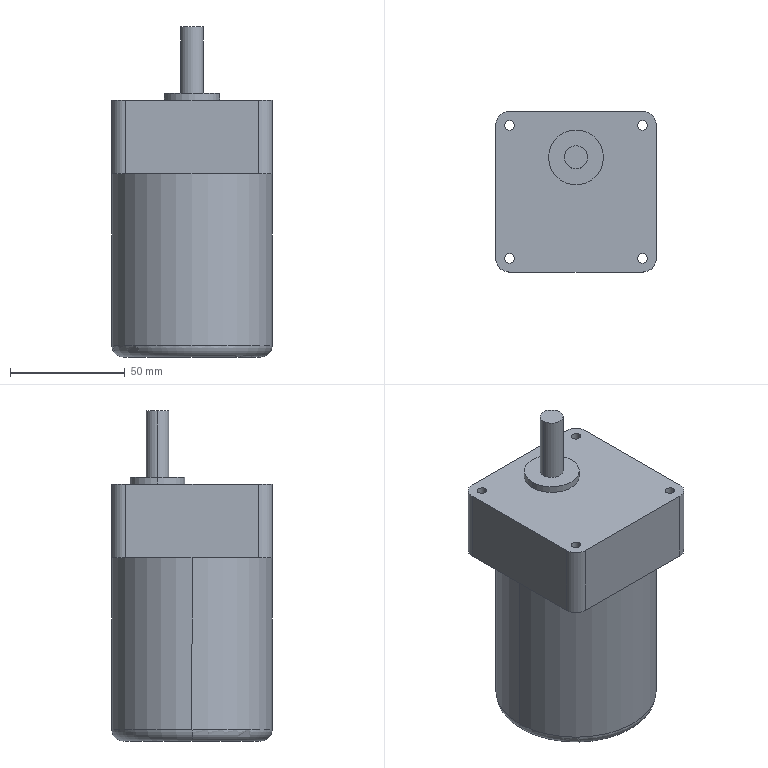Part | SolidWorks | features ICE 3, Fillet 2, Extrusion 1, HoleWzd 1 | 1 solid | 32 faces | box 70 x 70 x 144 mm | volume 464406 mm3 | cylinder 18 | plane 12 | torus 2 | commonest cylinder face diameters 4.2 x8 12 x4 10 x2 24 x2 70 x2
STEP:
#1=CARTESIAN_POINT('',(5.,15.,64.));
#2=VERTEX_POINT('',#1);
#3=CARTESIAN_POINT('',(-5.,15.,64.));
#4=VERTEX_POINT('',#3);
#5=CARTESIAN_POINT('',(0.,15.,64.));
#6=DIRECTION('',(0.,0.,1.));
#7=DIRECTION('',(1.,0.,0.));
#8=AXIS2_PLACEMENT_3D('',#5,#6,#7);
#9=CIRCLE('',#8,5.);
#10=EDGE_CURVE('',#2,#4,#9,.T.);
#11=ORIENTED_EDGE('',*,*,#10,.F.);
#12=CARTESIAN_POINT('',(5.,15.,35.));
#13=VERTEX_POINT('',#12);
#14=CARTESIAN_POINT('',(5.,15.,64.));
#15=DIRECTION('',(0.,0.,-1.));
#16=VECTOR('',#15,1000.);
#17=LINE('',#14,#16);
#18=EDGE_CURVE('',#2,#13,#17,.T.);
#19=ORIENTED_EDGE('',*,*,#18,.T.);
#20=CARTESIAN_POINT('',(-5.,15.,35.));
#21=VERTEX_POINT('',#20);
#22=CARTESIAN_POINT('',(0.,15.,35.));
#23=DIRECTION('',(0.,0.,1.));
#24=DIRECTION('',(1.,0.,0.));
#25=AXIS2_PLACEMENT_3D('',#22,#23,#24);
#26=CIRCLE('',#25,5.);
#27=EDGE_CURVE('',#13,#21,#26,.T.);
#28=ORIENTED_EDGE('',*,*,#27,.T.);
#29=CARTESIAN_POINT('',(-5.,15.,64.));
#30=DIRECTION('',(0.,0.,-1.));
#31=VECTOR('',#30,1000.);
#32=LINE('',#29,#31);
#33=EDGE_CURVE('',#4,#21,#32,.T.);
#34=ORIENTED_EDGE('',*,*,#33,.F.);
#35=EDGE_LOOP('',(#11,#19,#28,#34));
#36=FACE_OUTER_BOUND('',#35,.T.);
#37=CARTESIAN_POINT('',(0.,15.,64.));
#38=DIRECTION('',(0.,0.,-1.));
#39=DIRECTION('',(-1.,0.,0.));
#40=AXIS2_PLACEMENT_3D('',#37,#38,#39);
#41=CYLINDRICAL_SURFACE('',#40,5.);
#42=ADVANCED_FACE('',(#36),#41,.T.);
#43=CARTESIAN_POINT('',(12.,15.,35.));
#44=VERTEX_POINT('',#43);
#45=CARTESIAN_POINT('',(-12.,15.,35.));
#46=VERTEX_POINT('',#45);
#47=CARTESIAN_POINT('',(0.,15.,35.));
#48=DIRECTION('',(0.,0.,1.));
#49=DIRECTION('',(1.,0.,0.));
#50=AXIS2_PLACEMENT_3D('',#47,#48,#49);
#51=CIRCLE('',#50,12.);
#52=EDGE_CURVE('',#44,#46,#51,.T.);
#53=ORIENTED_EDGE('',*,*,#52,.F.);
#54=CARTESIAN_POINT('',(12.,15.,32.));
#55=VERTEX_POINT('',#54);
#56=CARTESIAN_POINT('',(12.,15.,35.));
#57=DIRECTION('',(0.,0.,-1.));
#58=VECTOR('',#57,1000.);
#59=LINE('',#56,#58);
#60=EDGE_CURVE('',#44,#55,#59,.T.);
#61=ORIENTED_EDGE('',*,*,#60,.T.);
#62=CARTESIAN_POINT('',(-12.,15.,32.));
#63=VERTEX_POINT('',#62);
#64=CARTESIAN_POINT('',(0.,15.,32.));
#65=DIRECTION('',(0.,0.,1.));
#66=DIRECTION('',(1.,0.,0.));
#67=AXIS2_PLACEMENT_3D('',#64,#65,#66);
#68=CIRCLE('',#67,12.);
#69=EDGE_CURVE('',#55,#63,#68,.T.);
#70=ORIENTED_EDGE('',*,*,#69,.T.);
#71=CARTESIAN_POINT('',(-12.,15.,35.));
#72=DIRECTION('',(0.,0.,-1.));
#73=VECTOR('',#72,1000.);
#74=LINE('',#71,#73);
#75=EDGE_CURVE('',#46,#63,#74,.T.);
#76=ORIENTED_EDGE('',*,*,#75,.F.);
#77=EDGE_LOOP('',(#53,#61,#70,#76));
#78=FACE_OUTER_BOUND('',#77,.T.);
#79=CARTESIAN_POINT('',(0.,15.,35.));
#80=DIRECTION('',(0.,0.,-1.));
#81=DIRECTION('',(-1.,0.,0.));
#82=AXIS2_PLACEMENT_3D('',#79,#80,#81);
#83=CYLINDRICAL_SURFACE('',#82,12.);
#84=ADVANCED_FACE('',(#78),#83,.T.);
#85=CARTESIAN_POINT('',(-31.091,28.991,0.));
#86=VERTEX_POINT('',#85);
#87=CARTESIAN_POINT('',(-26.891,28.991,0.));
#88=VERTEX_POINT('',#87);
#89=CARTESIAN_POINT('',(-28.991,28.991,0.));
#90=DIRECTION('',(0.,0.,1.));
#91=DIRECTION('',(1.,0.,0.));
#92=AXIS2_PLACEMENT_3D('',#89,#90,#91);
#93=CIRCLE('',#92,2.1);
#94=EDGE_CURVE('',#86,#88,#93,.T.);
#95=ORIENTED_EDGE('',*,*,#94,.F.);
#96=CARTESIAN_POINT('',(-31.091,28.991,32.));
#97=VERTEX_POINT('',#96);
#98=CARTESIAN_POINT('',(-31.091,28.991,32.));
#99=DIRECTION('',(0.,0.,1.));
#100=VECTOR('',#99,1000.);
#101=LINE('',#98,#100);
#102=EDGE_CURVE('',#86,#97,#101,.T.);
#103=ORIENTED_EDGE('',*,*,#102,.T.);
#104=CARTESIAN_POINT('',(-26.891,28.991,32.));
#105=VERTEX_POINT('',#104);
#106=CARTESIAN_POINT('',(-28.991,28.991,32.));
#107=DIRECTION('',(0.,0.,1.));
#108=DIRECTION('',(1.,0.,0.));
#109=AXIS2_PLACEMENT_3D('',#106,#107,#108);
#110=CIRCLE('',#109,2.1);
#111=EDGE_CURVE('',#97,#105,#110,.T.);
#112=ORIENTED_EDGE('',*,*,#111,.T.);
#113=CARTESIAN_POINT('',(-26.891,28.991,32.));
#114=DIRECTION('',(0.,0.,1.));
#115=VECTOR('',#114,1000.);
#116=LINE('',#113,#115);
#117=EDGE_CURVE('',#88,#105,#116,.T.);
#118=ORIENTED_EDGE('',*,*,#117,.F.);
#119=EDGE_LOOP('',(#95,#103,#112,#118));
#120=FACE_OUTER_BOUND('',#119,.T.);
#121=CARTESIAN_POINT('',(-28.991,28.991,32.));
#122=DIRECTION('',(0.,0.,1.));
#123=DIRECTION('',(1.,0.,0.));
#124=AXIS2_PLACEMENT_3D('',#121,#122,#123);
#125=CYLINDRICAL_SURFACE('',#124,2.1);
#126=ADVANCED_FACE('',(#120),#125,.F.);
#127=CARTESIAN_POINT('',(-31.091,-28.991,0.));
#128=VERTEX_POINT('',#127);
#129=CARTESIAN_POINT('',(-26.891,-28.991,0.));
#130=VERTEX_POINT('',#129);
#131=CARTESIAN_POINT('',(-28.991,-28.991,0.));
#132=DIRECTION('',(0.,0.,1.));
#133=DIRECTION('',(1.,0.,0.));
#134=AXIS2_PLACEMENT_3D('',#131,#132,#133);
#135=CIRCLE('',#134,2.1);
#136=EDGE_CURVE('',#128,#130,#135,.T.);
#137=ORIENTED_EDGE('',*,*,#136,.F.);
#138=CARTESIAN_POINT('',(-31.091,-28.991,32.));
#139=VERTEX_POINT('',#138);
#140=CARTESIAN_POINT('',(-31.091,-28.991,32.));
#141=DIRECTION('',(0.,0.,1.));
#142=VECTOR('',#141,1000.);
#143=LINE('',#140,#142);
#144=EDGE_CURVE('',#128,#139,#143,.T.);
#145=ORIENTED_EDGE('',*,*,#144,.T.);
#146=CARTESIAN_POINT('',(-26.891,-28.991,32.));
#147=VERTEX_POINT('',#146);
#148=CARTESIAN_POINT('',(-28.991,-28.991,32.));
#149=DIRECTION('',(0.,0.,1.));
#150=DIRECTION('',(1.,0.,0.));
#151=AXIS2_PLACEMENT_3D('',#148,#149,#150);
#152=CIRCLE('',#151,2.1);
#153=EDGE_CURVE('',#139,#147,#152,.T.);
#154=ORIENTED_EDGE('',*,*,#153,.T.);
#155=CARTESIAN_POINT('',(-26.891,-28.991,32.));
#156=DIRECTION('',(0.,0.,1.));
#157=VECTOR('',#156,1000.);
#158=LINE('',#155,#157);
#159=EDGE_CURVE('',#130,#147,#158,.T.);
#160=ORIENTED_EDGE('',*,*,#159,.F.);
#161=EDGE_LOOP('',(#137,#145,#154,#160));
#162=FACE_OUTER_BOUND('',#161,.T.);
#163=CARTESIAN_POINT('',(-28.991,-28.991,32.));
#164=DIRECTION('',(0.,0.,1.));
#165=DIRECTION('',(1.,0.,0.));
#166=AXIS2_PLACEMENT_3D('',#163,#164,#165);
#167=CYLINDRICAL_SURFACE('',#166,2.1);
#168=ADVANCED_FACE('',(#162),#167,.F.);
#169=CARTESIAN_POINT('',(26.891,-28.991,0.));
#170=VERTEX_POINT('',#169);
#171=CARTESIAN_POINT('',(31.091,-28.991,0.));
#172=VERTEX_POINT('',#171);
#173=CARTESIAN_POINT('',(28.991,-28.991,0.));
#174=DIRECTION('',(0.,0.,1.));
#175=DIRECTION('',(1.,0.,0.));
#176=AXIS2_PLACEMENT_3D('',#173,#174,#175);
#177=CIRCLE('',#176,2.1);
#178=EDGE_CURVE('',#170,#172,#177,.T.);
#179=ORIENTED_EDGE('',*,*,#178,.F.);
#180=CARTESIAN_POINT('',(26.891,-28.991,32.));
#181=VERTEX_POINT('',#180);
#182=CARTESIAN_POINT('',(26.891,-28.991,32.));
#183=DIRECTION('',(0.,0.,1.));
#184=VECTOR('',#183,1000.);
#185=LINE('',#182,#184);
#186=EDGE_CURVE('',#170,#181,#185,.T.);
#187=ORIENTED_EDGE('',*,*,#186,.T.);
#188=CARTESIAN_POINT('',(31.091,-28.991,32.));
#189=VERTEX_POINT('',#188);
#190=CARTESIAN_POINT('',(28.991,-28.991,32.));
#191=DIRECTION('',(0.,0.,1.));
#192=DIRECTION('',(1.,0.,0.));
#193=AXIS2_PLACEMENT_3D('',#190,#191,#192);
#194=CIRCLE('',#193,2.1);
#195=EDGE_CURVE('',#181,#189,#194,.T.);
#196=ORIENTED_EDGE('',*,*,#195,.T.);
#197=CARTESIAN_POINT('',(31.091,-28.991,32.));
#198=DIRECTION('',(0.,0.,1.));
#199=VECTOR('',#198,1000.);
#200=LINE('',#197,#199);
#201=EDGE_CURVE('',#172,#189,#200,.T.);
#202=ORIENTED_EDGE('',*,*,#201,.F.);
#203=EDGE_LOOP('',(#179,#187,#196,#202));
#204=FACE_OUTER_BOUND('',#203,.T.);
#205=CARTESIAN_POINT('',(28.991,-28.991,32.));
#206=DIRECTION('',(0.,0.,1.));
#207=DIRECTION('',(1.,0.,0.));
#208=AXIS2_PLACEMENT_3D('',#205,#206,#207);
#209=CYLINDRICAL_SURFACE('',#208,2.1);
#210=ADVANCED_FACE('',(#204),#209,.F.);
#211=CARTESIAN_POINT('',(26.891,28.991,0.));
#212=VERTEX_POINT('',#211);
#213=CARTESIAN_POINT('',(31.091,28.991,0.));
#214=VERTEX_POINT('',#213);
#215=CARTESIAN_POINT('',(28.991,28.991,0.));
#216=DIRECTION('',(0.,0.,1.));
#217=DIRECTION('',(1.,0.,0.));
#218=AXIS2_PLACEMENT_3D('',#215,#216,#217);
#219=CIRCLE('',#218,2.1);
#220=EDGE_CURVE('',#212,#214,#219,.T.);
#221=ORIENTED_EDGE('',*,*,#220,.F.);
#222=CARTESIAN_POINT('',(26.891,28.991,32.));
#223=VERTEX_POINT('',#222);
#224=CARTESIAN_POINT('',(26.891,28.991,32.));
#225=DIRECTION('',(0.,0.,1.));
#226=VECTOR('',#225,1000.);
#227=LINE('',#224,#226);
#228=EDGE_CURVE('',#212,#223,#227,.T.);
#229=ORIENTED_EDGE('',*,*,#228,.T.);
#230=CARTESIAN_POINT('',(31.091,28.991,32.));
#231=VERTEX_POINT('',#230);
#232=CARTESIAN_POINT('',(28.991,28.991,32.));
#233=DIRECTION('',(0.,0.,1.));
#234=DIRECTION('',(1.,0.,0.));
#235=AXIS2_PLACEMENT_3D('',#232,#233,#234);
#236=CIRCLE('',#235,2.1);
#237=EDGE_CURVE('',#223,#231,#236,.T.);
#238=ORIENTED_EDGE('',*,*,#237,.T.);
#239=CARTESIAN_POINT('',(31.091,28.991,32.));
#240=DIRECTION('',(0.,0.,1.));
#241=VECTOR('',#240,1000.);
#242=LINE('',#239,#241);
#243=EDGE_CURVE('',#214,#231,#242,.T.);
#244=ORIENTED_EDGE('',*,*,#243,.F.);
#245=EDGE_LOOP('',(#221,#229,#238,#244));
#246=FACE_OUTER_BOUND('',#245,.T.);
#247=CARTESIAN_POINT('',(28.991,28.991,32.));
#248=DIRECTION('',(0.,0.,1.));
#249=DIRECTION('',(1.,0.,0.));
#250=AXIS2_PLACEMENT_3D('',#247,#248,#249);
#251=CYLINDRICAL_SURFACE('',#250,2.1);
#252=ADVANCED_FACE('',(#246),#251,.F.);
#253=CARTESIAN_POINT('',(35.,0.,-75.));
#254=VERTEX_POINT('',#253);
#255=CARTESIAN_POINT('',(-35.,0.,-75.));
#256=VERTEX_POINT('',#255);
#257=CARTESIAN_POINT('',(0.,0.,-75.));
#258=DIRECTION('',(0.,0.,1.));
#259=DIRECTION('',(-1.,0.,0.));
#260=AXIS2_PLACEMENT_3D('',#257,#258,#259);
#261=CIRCLE('',#260,35.);
#262=EDGE_CURVE('',#254,#256,#261,.T.);
#263=ORIENTED_EDGE('',*,*,#262,.F.);
#264=CARTESIAN_POINT('',(30.,0.,-80.));
#265=VERTEX_POINT('',#264);
#266=CARTESIAN_POINT('',(30.,0.,-75.));
#267=DIRECTION('',(0.,1.,0.));
#268=DIRECTION('',(-1.,0.,0.));
#269=AXIS2_PLACEMENT_3D('',#266,#267,#268);
#270=CIRCLE('',#269,5.);
#271=EDGE_CURVE('',#254,#265,#270,.T.);
#272=ORIENTED_EDGE('',*,*,#271,.T.);
#273=CARTESIAN_POINT('',(-30.,0.,-80.));
#274=VERTEX_POINT('',#273);
#275=CARTESIAN_POINT('',(0.,0.,-80.));
#276=DIRECTION('',(0.,0.,-1.));
#277=DIRECTION('',(-1.,0.,0.));
#278=AXIS2_PLACEMENT_3D('',#275,#276,#277);
#279=CIRCLE('',#278,30.);
#280=EDGE_CURVE('',#274,#265,#279,.T.);
#281=ORIENTED_EDGE('',*,*,#280,.F.);
#282=CARTESIAN_POINT('',(-30.,0.,-75.));
#283=DIRECTION('',(0.,-1.,0.));
#284=DIRECTION('',(0.,0.,-1.));
#285=AXIS2_PLACEMENT_3D('',#282,#283,#284);
#286=CIRCLE('',#285,5.);
#287=EDGE_CURVE('',#256,#274,#286,.T.);
#288=ORIENTED_EDGE('',*,*,#287,.F.);
#289=EDGE_LOOP('',(#263,#272,#281,#288));
#290=FACE_OUTER_BOUND('',#289,.T.);
#291=CARTESIAN_POINT('',(0.,0.,-75.));
#292=DIRECTION('',(0.,0.,-1.));
#293=DIRECTION('',(-1.,0.,0.));
#294=AXIS2_PLACEMENT_3D('',#291,#292,#293);
#295=TOROIDAL_SURFACE('',#294,30.,5.);
#296=ADVANCED_FACE('',(#290),#295,.T.);
#297=ORIENTED_EDGE('',*,*,#262,.T.);
#298=CARTESIAN_POINT('',(-35.,0.,0.));
#299=VERTEX_POINT('',#298);
#300=CARTESIAN_POINT('',(-35.,0.,-80.));
#301=DIRECTION('',(0.,0.,1.));
#302=VECTOR('',#301,1000.);
#303=LINE('',#300,#302);
#304=EDGE_CURVE('',#256,#299,#303,.T.);
#305=ORIENTED_EDGE('',*,*,#304,.T.);
#306=CARTESIAN_POINT('',(0.,35.,0.));
#307=VERTEX_POINT('',#306);
#308=CARTESIAN_POINT('',(0.,0.,0.));
#309=DIRECTION('',(0.,0.,-1.));
#310=DIRECTION('',(-1.,0.,0.));
#311=AXIS2_PLACEMENT_3D('',#308,#309,#310);
#312=CIRCLE('',#311,35.);
#313=EDGE_CURVE('',#299,#307,#312,.T.);
#314=ORIENTED_EDGE('',*,*,#313,.T.);
#315=CARTESIAN_POINT('',(35.,0.,0.));
#316=VERTEX_POINT('',#315);
#317=CARTESIAN_POINT('',(0.,0.,0.));
#318=DIRECTION('',(0.,0.,-1.));
#319=DIRECTION('',(-1.,0.,0.));
#320=AXIS2_PLACEMENT_3D('',#317,#318,#319);
#321=CIRCLE('',#320,35.);
#322=EDGE_CURVE('',#307,#316,#321,.T.);
#323=ORIENTED_EDGE('',*,*,#322,.T.);
#324=CARTESIAN_POINT('',(35.,0.,-80.));
#325=DIRECTION('',(0.,0.,1.));
#326=VECTOR('',#325,1000.);
#327=LINE('',#324,#326);
#328=EDGE_CURVE('',#254,#316,#327,.T.);
#329=ORIENTED_EDGE('',*,*,#328,.F.);
#330=EDGE_LOOP('',(#297,#305,#314,#323,#329));
#331=FACE_OUTER_BOUND('',#330,.T.);
#332=CARTESIAN_POINT('',(0.,0.,-80.));
#333=DIRECTION('',(0.,0.,1.));
#334=DIRECTION('',(1.,0.,0.));
#335=AXIS2_PLACEMENT_3D('',#332,#333,#334);
#336=CYLINDRICAL_SURFACE('',#335,35.);
#337=ADVANCED_FACE('',(#331),#336,.T.);
#338=CARTESIAN_POINT('',(-35.,29.,32.));
#339=VERTEX_POINT('',#338);
#340=CARTESIAN_POINT('',(-35.,-29.,32.));
#341=VERTEX_POINT('',#340);
#342=CARTESIAN_POINT('',(-35.,35.,32.));
#343=DIRECTION('',(0.,-1.,0.));
#344=VECTOR('',#343,1000.);
#345=LINE('',#342,#344);
#346=EDGE_CURVE('',#339,#341,#345,.T.);
#347=ORIENTED_EDGE('',*,*,#346,.T.);
#348=CARTESIAN_POINT('',(-29.,-35.,32.));
#349=VERTEX_POINT('',#348);
#350=CARTESIAN_POINT('',(-29.,-29.,32.));
#351=DIRECTION('',(0.,0.,1.));
#352=DIRECTION('',(1.,0.,0.));
#353=AXIS2_PLACEMENT_3D('',#350,#351,#352);
#354=CIRCLE('',#353,6.);
#355=EDGE_CURVE('',#341,#349,#354,.T.);
#356=ORIENTED_EDGE('',*,*,#355,.T.);
#357=CARTESIAN_POINT('',(29.,-35.,32.));
#358=VERTEX_POINT('',#357);
#359=CARTESIAN_POINT('',(-35.,-35.,32.));
#360=DIRECTION('',(1.,0.,0.));
#361=VECTOR('',#360,1000.);
#362=LINE('',#359,#361);
#363=EDGE_CURVE('',#349,#358,#362,.T.);
#364=ORIENTED_EDGE('',*,*,#363,.T.);
#365=CARTESIAN_POINT('',(35.,-29.,32.));
#366=VERTEX_POINT('',#365);
#367=CARTESIAN_POINT('',(29.,-29.,32.));
#368=DIRECTION('',(0.,0.,1.));
#369=DIRECTION('',(1.,0.,0.));
#370=AXIS2_PLACEMENT_3D('',#367,#368,#369);
#371=CIRCLE('',#370,6.);
#372=EDGE_CURVE('',#358,#366,#371,.T.);
#373=ORIENTED_EDGE('',*,*,#372,.T.);
#374=CARTESIAN_POINT('',(35.,29.,32.));
#375=VERTEX_POINT('',#374);
#376=CARTESIAN_POINT('',(35.,35.,32.));
#377=DIRECTION('',(0.,1.,0.));
#378=VECTOR('',#377,1000.);
#379=LINE('',#376,#378);
#380=EDGE_CURVE('',#366,#375,#379,.T.);
#381=ORIENTED_EDGE('',*,*,#380,.T.);
#382=CARTESIAN_POINT('',(29.,35.,32.));
#383=VERTEX_POINT('',#382);
#384=CARTESIAN_POINT('',(29.,29.,32.));
#385=DIRECTION('',(0.,0.,1.));
#386=DIRECTION('',(1.,0.,0.));
#387=AXIS2_PLACEMENT_3D('',#384,#385,#386);
#388=CIRCLE('',#387,6.);
#389=EDGE_CURVE('',#375,#383,#388,.T.);
#390=ORIENTED_EDGE('',*,*,#389,.T.);
#391=CARTESIAN_POINT('',(-29.,35.,32.));
#392=VERTEX_POINT('',#391);
#393=CARTESIAN_POINT('',(-35.,35.,32.));
#394=DIRECTION('',(-1.,0.,0.));
#395=VECTOR('',#394,1000.);
#396=LINE('',#393,#395);
#397=EDGE_CURVE('',#383,#392,#396,.T.);
#398=ORIENTED_EDGE('',*,*,#397,.T.);
#399=CARTESIAN_POINT('',(-29.,29.,32.));
#400=DIRECTION('',(0.,0.,1.));
#401=DIRECTION('',(1.,0.,0.));
#402=AXIS2_PLACEMENT_3D('',#399,#400,#401);
#403=CIRCLE('',#402,6.);
#404=EDGE_CURVE('',#392,#339,#403,.T.);
#405=ORIENTED_EDGE('',*,*,#404,.T.);
#406=EDGE_LOOP('',(#347,#356,#364,#373,#381,#390,#398,#405));
#407=FACE_OUTER_BOUND('',#406,.T.);
#408=CARTESIAN_POINT('',(28.991,28.991,32.));
#409=DIRECTION('',(0.,0.,1.));
#410=DIRECTION('',(1.,0.,0.));
#411=AXIS2_PLACEMENT_3D('',#408,#409,#410);
#412=CIRCLE('',#411,2.1);
#413=EDGE_CURVE('',#231,#223,#412,.T.);
#414=ORIENTED_EDGE('',*,*,#413,.F.);
#415=ORIENTED_EDGE('',*,*,#237,.F.);
#416=EDGE_LOOP('',(#414,#415));
#417=FACE_BOUND('',#416,.T.);
#418=CARTESIAN_POINT('',(28.991,-28.991,32.));
#419=DIRECTION('',(0.,0.,1.));
#420=DIRECTION('',(1.,0.,0.));
#421=AXIS2_PLACEMENT_3D('',#418,#419,#420);
#422=CIRCLE('',#421,2.1);
#423=EDGE_CURVE('',#189,#181,#422,.T.);
#424=ORIENTED_EDGE('',*,*,#423,.F.);
#425=ORIENTED_EDGE('',*,*,#195,.F.);
#426=EDGE_LOOP('',(#424,#425));
#427=FACE_BOUND('',#426,.T.);
#428=CARTESIAN_POINT('',(-28.991,-28.991,32.));
#429=DIRECTION('',(0.,0.,1.));
#430=DIRECTION('',(1.,0.,0.));
#431=AXIS2_PLACEMENT_3D('',#428,#429,#430);
#432=CIRCLE('',#431,2.1);
#433=EDGE_CURVE('',#147,#139,#432,.T.);
#434=ORIENTED_EDGE('',*,*,#433,.F.);
#435=ORIENTED_EDGE('',*,*,#153,.F.);
#436=EDGE_LOOP('',(#434,#435));
#437=FACE_BOUND('',#436,.T.);
#438=CARTESIAN_POINT('',(-28.991,28.991,32.));
#439=DIRECTION('',(0.,0.,1.));
#440=DIRECTION('',(1.,0.,0.));
#441=AXIS2_PLACEMENT_3D('',#438,#439,#440);
#442=CIRCLE('',#441,2.1);
#443=EDGE_CURVE('',#105,#97,#442,.T.);
#444=ORIENTED_EDGE('',*,*,#443,.F.);
#445=ORIENTED_EDGE('',*,*,#111,.F.);
#446=EDGE_LOOP('',(#444,#445));
#447=FACE_BOUND('',#446,.T.);
#448=CARTESIAN_POINT('',(0.,15.,32.));
#449=DIRECTION('',(0.,0.,1.));
#450=DIRECTION('',(1.,0.,0.));
#451=AXIS2_PLACEMENT_3D('',#448,#449,#450);
#452=CIRCLE('',#451,12.);
#453=EDGE_CURVE('',#63,#55,#452,.T.);
#454=ORIENTED_EDGE('',*,*,#453,.F.);
#455=ORIENTED_EDGE('',*,*,#69,.F.);
#456=EDGE_LOOP('',(#454,#455));
#457=FACE_BOUND('',#456,.T.);
#458=CARTESIAN_POINT('',(0.,0.,32.));
#459=DIRECTION('',(0.,0.,1.));
#460=DIRECTION('',(1.,0.,0.));
#461=AXIS2_PLACEMENT_3D('',#458,#459,#460);
#462=PLANE('',#461);
#463=ADVANCED_FACE('',(#407,#417,#427,#437,#447,#457),#462,.T.);
#464=CARTESIAN_POINT('',(-28.991,28.991,0.));
#465=DIRECTION('',(0.,0.,1.));
#466=DIRECTION('',(1.,0.,0.));
#467=AXIS2_PLACEMENT_3D('',#464,#465,#466);
#468=CIRCLE('',#467,2.1);
#469=EDGE_CURVE('',#88,#86,#468,.T.);
#470=ORIENTED_EDGE('',*,*,#469,.T.);
#471=ORIENTED_EDGE('',*,*,#94,.T.);
#472=EDGE_LOOP('',(#470,#471));
#473=FACE_BOUND('',#472,.T.);
#474=CARTESIAN_POINT('',(-35.,29.,0.));
#475=VERTEX_POINT('',#474);
#476=CARTESIAN_POINT('',(-35.,35.,0.));
#477=DIRECTION('',(0.,-1.,0.));
#478=VECTOR('',#477,1000.);
#479=LINE('',#476,#478);
#480=EDGE_CURVE('',#475,#299,#479,.T.);
#481=ORIENTED_EDGE('',*,*,#480,.F.);
#482=CARTESIAN_POINT('',(-29.,35.,0.));
#483=VERTEX_POINT('',#482);
#484=CARTESIAN_POINT('',(-29.,29.,0.));
#485=DIRECTION('',(0.,0.,-1.));
#486=DIRECTION('',(1.,0.,0.));
#487=AXIS2_PLACEMENT_3D('',#484,#485,#486);
#488=CIRCLE('',#487,6.);
#489=EDGE_CURVE('',#475,#483,#488,.T.);
#490=ORIENTED_EDGE('',*,*,#489,.T.);
#491=CARTESIAN_POINT('',(-35.,35.,0.));
#492=DIRECTION('',(-1.,0.,0.));
#493=VECTOR('',#492,1000.);
#494=LINE('',#491,#493);
#495=EDGE_CURVE('',#307,#483,#494,.T.);
#496=ORIENTED_EDGE('',*,*,#495,.F.);
#497=ORIENTED_EDGE('',*,*,#313,.F.);
#498=EDGE_LOOP('',(#481,#490,#496,#497));
#499=FACE_OUTER_BOUND('',#498,.T.);
#500=CARTESIAN_POINT('',(0.,0.,0.));
#501=DIRECTION('',(0.,0.,1.));
#502=DIRECTION('',(1.,0.,0.));
#503=AXIS2_PLACEMENT_3D('',#500,#501,#502);
#504=PLANE('',#503);
#505=ADVANCED_FACE('',(#473,#499),#504,.F.);
#506=CARTESIAN_POINT('',(28.991,28.991,0.));
#507=DIRECTION('',(0.,0.,1.));
#508=DIRECTION('',(1.,0.,0.));
#509=AXIS2_PLACEMENT_3D('',#506,#507,#508);
#510=CIRCLE('',#509,2.1);
#511=EDGE_CURVE('',#214,#212,#510,.T.);
#512=ORIENTED_EDGE('',*,*,#511,.T.);
#513=ORIENTED_EDGE('',*,*,#220,.T.);
#514=EDGE_LOOP('',(#512,#513));
#515=FACE_BOUND('',#514,.T.);
#516=CARTESIAN_POINT('',(29.,35.,0.));
#517=VERTEX_POINT('',#516);
#518=CARTESIAN_POINT('',(-35.,35.,0.));
#519=DIRECTION('',(-1.,0.,0.));
#520=VECTOR('',#519,1000.);
#521=LINE('',#518,#520);
#522=EDGE_CURVE('',#517,#307,#521,.T.);
#523=ORIENTED_EDGE('',*,*,#522,.F.);
#524=CARTESIAN_POINT('',(35.,29.,0.));
#525=VERTEX_POINT('',#524);
#526=CARTESIAN_POINT('',(29.,29.,0.));
#527=DIRECTION('',(0.,0.,-1.));
#528=DIRECTION('',(1.,0.,0.));
#529=AXIS2_PLACEMENT_3D('',#526,#527,#528);
#530=CIRCLE('',#529,6.);
#531=EDGE_CURVE('',#517,#525,#530,.T.);
#532=ORIENTED_EDGE('',*,*,#531,.T.);
#533=CARTESIAN_POINT('',(35.,35.,0.));
#534=DIRECTION('',(0.,1.,0.));
#535=VECTOR('',#534,1000.);
#536=LINE('',#533,#535);
#537=EDGE_CURVE('',#316,#525,#536,.T.);
#538=ORIENTED_EDGE('',*,*,#537,.F.);
#539=ORIENTED_EDGE('',*,*,#322,.F.);
#540=EDGE_LOOP('',(#523,#532,#538,#539));
#541=FACE_OUTER_BOUND('',#540,.T.);
#542=CARTESIAN_POINT('',(0.,0.,0.));
#543=DIRECTION('',(0.,0.,1.));
#544=DIRECTION('',(1.,0.,0.));
#545=AXIS2_PLACEMENT_3D('',#542,#543,#544);
#546=PLANE('',#545);
#547=ADVANCED_FACE('',(#515,#541),#546,.F.);
#548=CARTESIAN_POINT('',(28.991,-28.991,0.));
#549=DIRECTION('',(0.,0.,1.));
#550=DIRECTION('',(1.,0.,0.));
#551=AXIS2_PLACEMENT_3D('',#548,#549,#550);
#552=CIRCLE('',#551,2.1);
#553=EDGE_CURVE('',#172,#170,#552,.T.);
#554=ORIENTED_EDGE('',*,*,#553,.T.);
#555=ORIENTED_EDGE('',*,*,#178,.T.);
#556=EDGE_LOOP('',(#554,#555));
#557=FACE_BOUND('',#556,.T.);
#558=CARTESIAN_POINT('',(35.,-29.,0.));
#559=VERTEX_POINT('',#558);
#560=CARTESIAN_POINT('',(35.,35.,0.));
#561=DIRECTION('',(0.,1.,0.));
#562=VECTOR('',#561,1000.);
#563=LINE('',#560,#562);
#564=EDGE_CURVE('',#559,#316,#563,.T.);
#565=ORIENTED_EDGE('',*,*,#564,.F.);
#566=CARTESIAN_POINT('',(29.,-35.,0.));
#567=VERTEX_POINT('',#566);
#568=CARTESIAN_POINT('',(29.,-29.,0.));
#569=DIRECTION('',(0.,0.,-1.));
#570=DIRECTION('',(1.,0.,0.));
#571=AXIS2_PLACEMENT_3D('',#568,#569,#570);
#572=CIRCLE('',#571,6.);
#573=EDGE_CURVE('',#559,#567,#572,.T.);
#574=ORIENTED_EDGE('',*,*,#573,.T.);
#575=CARTESIAN_POINT('',(0.,-35.,0.));
#576=VERTEX_POINT('',#575);
#577=CARTESIAN_POINT('',(-35.,-35.,0.));
#578=DIRECTION('',(1.,0.,0.));
#579=VECTOR('',#578,1000.);
#580=LINE('',#577,#579);
#581=EDGE_CURVE('',#576,#567,#580,.T.);
#582=ORIENTED_EDGE('',*,*,#581,.F.);
#583=CARTESIAN_POINT('',(0.,0.,0.));
#584=DIRECTION('',(0.,0.,-1.));
#585=DIRECTION('',(-1.,0.,0.));
#586=AXIS2_PLACEMENT_3D('',#583,#584,#585);
#587=CIRCLE('',#586,35.);
#588=EDGE_CURVE('',#316,#576,#587,.T.);
#589=ORIENTED_EDGE('',*,*,#588,.F.);
#590=EDGE_LOOP('',(#565,#574,#582,#589));
#591=FACE_OUTER_BOUND('',#590,.T.);
#592=CARTESIAN_POINT('',(0.,0.,0.));
#593=DIRECTION('',(0.,0.,1.));
#594=DIRECTION('',(1.,0.,0.));
#595=AXIS2_PLACEMENT_3D('',#592,#593,#594);
#596=PLANE('',#595);
#597=ADVANCED_FACE('',(#557,#591),#596,.F.);
#598=CARTESIAN_POINT('',(-28.991,-28.991,0.));
#599=DIRECTION('',(0.,0.,1.));
#600=DIRECTION('',(1.,0.,0.));
#601=AXIS2_PLACEMENT_3D('',#598,#599,#600);
#602=CIRCLE('',#601,2.1);
#603=EDGE_CURVE('',#130,#128,#602,.T.);
#604=ORIENTED_EDGE('',*,*,#603,.T.);
#605=ORIENTED_EDGE('',*,*,#136,.T.);
#606=EDGE_LOOP('',(#604,#605));
#607=FACE_BOUND('',#606,.T.);
#608=CARTESIAN_POINT('',(-29.,-35.,0.));
#609=VERTEX_POINT('',#608);
#610=CARTESIAN_POINT('',(-35.,-35.,0.));
#611=DIRECTION('',(1.,0.,0.));
#612=VECTOR('',#611,1000.);
#613=LINE('',#610,#612);
#614=EDGE_CURVE('',#609,#576,#613,.T.);
#615=ORIENTED_EDGE('',*,*,#614,.F.);
#616=CARTESIAN_POINT('',(-35.,-29.,0.));
#617=VERTEX_POINT('',#616);
#618=CARTESIAN_POINT('',(-29.,-29.,0.));
#619=DIRECTION('',(0.,0.,-1.));
#620=DIRECTION('',(1.,0.,0.));
#621=AXIS2_PLACEMENT_3D('',#618,#619,#620);
#622=CIRCLE('',#621,6.);
#623=EDGE_CURVE('',#609,#617,#622,.T.);
#624=ORIENTED_EDGE('',*,*,#623,.T.);
#625=CARTESIAN_POINT('',(-35.,35.,0.));
#626=DIRECTION('',(0.,-1.,0.));
#627=VECTOR('',#626,1000.);
#628=LINE('',#625,#627);
#629=EDGE_CURVE('',#299,#617,#628,.T.);
#630=ORIENTED_EDGE('',*,*,#629,.F.);
#631=CARTESIAN_POINT('',(0.,0.,0.));
#632=DIRECTION('',(0.,0.,-1.));
#633=DIRECTION('',(-1.,0.,0.));
#634=AXIS2_PLACEMENT_3D('',#631,#632,#633);
#635=CIRCLE('',#634,35.);
#636=EDGE_CURVE('',#576,#299,#635,.T.);
#637=ORIENTED_EDGE('',*,*,#636,.F.);
#638=EDGE_LOOP('',(#615,#624,#630,#637));
#639=FACE_OUTER_BOUND('',#638,.T.);
#640=CARTESIAN_POINT('',(0.,0.,0.));
#641=DIRECTION('',(0.,0.,1.));
#642=DIRECTION('',(1.,0.,0.));
#643=AXIS2_PLACEMENT_3D('',#640,#641,#642);
#644=PLANE('',#643);
#645=ADVANCED_FACE('',(#607,#639),#644,.F.);
#646=ORIENTED_EDGE('',*,*,#380,.F.);
#647=CARTESIAN_POINT('',(35.,-29.,32.));
#648=DIRECTION('',(0.,0.,-1.));
#649=VECTOR('',#648,1000.);
#650=LINE('',#647,#649);
#651=EDGE_CURVE('',#366,#559,#650,.T.);
#652=ORIENTED_EDGE('',*,*,#651,.T.);
#653=ORIENTED_EDGE('',*,*,#564,.T.);
#654=ORIENTED_EDGE('',*,*,#537,.T.);
#655=CARTESIAN_POINT('',(35.,29.,32.));
#656=DIRECTION('',(0.,0.,1.));
#657=VECTOR('',#656,1000.);
#658=LINE('',#655,#657);
#659=EDGE_CURVE('',#525,#375,#658,.T.);
#660=ORIENTED_EDGE('',*,*,#659,.T.);
#661=EDGE_LOOP('',(#646,#652,#653,#654,#660));
#662=FACE_OUTER_BOUND('',#661,.T.);
#663=CARTESIAN_POINT('',(35.,35.,32.));
#664=DIRECTION('',(-1.,0.,0.));
#665=DIRECTION('',(0.,-1.,0.));
#666=AXIS2_PLACEMENT_3D('',#663,#664,#665);
#667=PLANE('',#666);
#668=ADVANCED_FACE('',(#662),#667,.F.);
#669=ORIENTED_EDGE('',*,*,#495,.T.);
#670=CARTESIAN_POINT('',(-29.,35.,32.));
#671=DIRECTION('',(0.,0.,1.));
#672=VECTOR('',#671,1000.);
#673=LINE('',#670,#672);
#674=EDGE_CURVE('',#483,#392,#673,.T.);
#675=ORIENTED_EDGE('',*,*,#674,.T.);
#676=ORIENTED_EDGE('',*,*,#397,.F.);
#677=CARTESIAN_POINT('',(29.,35.,32.));
#678=DIRECTION('',(0.,0.,-1.));
#679=VECTOR('',#678,1000.);
#680=LINE('',#677,#679);
#681=EDGE_CURVE('',#383,#517,#680,.T.);
#682=ORIENTED_EDGE('',*,*,#681,.T.);
#683=ORIENTED_EDGE('',*,*,#522,.T.);
#684=EDGE_LOOP('',(#669,#675,#676,#682,#683));
#685=FACE_OUTER_BOUND('',#684,.T.);
#686=CARTESIAN_POINT('',(-35.,35.,32.));
#687=DIRECTION('',(0.,-1.,0.));
#688=DIRECTION('',(0.,0.,-1.));
#689=AXIS2_PLACEMENT_3D('',#686,#687,#688);
#690=PLANE('',#689);
#691=ADVANCED_FACE('',(#685),#690,.F.);
#692=ORIENTED_EDGE('',*,*,#629,.T.);
#693=CARTESIAN_POINT('',(-35.,-29.,32.));
#694=DIRECTION('',(0.,0.,1.));
#695=VECTOR('',#694,1000.);
#696=LINE('',#693,#695);
#697=EDGE_CURVE('',#617,#341,#696,.T.);
#698=ORIENTED_EDGE('',*,*,#697,.T.);
#699=ORIENTED_EDGE('',*,*,#346,.F.);
#700=CARTESIAN_POINT('',(-35.,29.,32.));
#701=DIRECTION('',(0.,0.,-1.));
#702=VECTOR('',#701,1000.);
#703=LINE('',#700,#702);
#704=EDGE_CURVE('',#339,#475,#703,.T.);
#705=ORIENTED_EDGE('',*,*,#704,.T.);
#706=ORIENTED_EDGE('',*,*,#480,.T.);
#707=EDGE_LOOP('',(#692,#698,#699,#705,#706));
#708=FACE_OUTER_BOUND('',#707,.T.);
#709=CARTESIAN_POINT('',(-35.,35.,32.));
#710=DIRECTION('',(1.,0.,0.));
#711=DIRECTION('',(0.,1.,0.));
#712=AXIS2_PLACEMENT_3D('',#709,#710,#711);
#713=PLANE('',#712);
#714=ADVANCED_FACE('',(#708),#713,.F.);
#715=ORIENTED_EDGE('',*,*,#363,.F.);
#716=CARTESIAN_POINT('',(-29.,-35.,32.));
#717=DIRECTION('',(0.,0.,-1.));
#718=VECTOR('',#717,1000.);
#719=LINE('',#716,#718);
#720=EDGE_CURVE('',#349,#609,#719,.T.);
#721=ORIENTED_EDGE('',*,*,#720,.T.);
#722=ORIENTED_EDGE('',*,*,#614,.T.);
#723=ORIENTED_EDGE('',*,*,#581,.T.);
#724=CARTESIAN_POINT('',(29.,-35.,32.));
#725=DIRECTION('',(0.,0.,1.));
#726=VECTOR('',#725,1000.);
#727=LINE('',#724,#726);
#728=EDGE_CURVE('',#567,#358,#727,.T.);
#729=ORIENTED_EDGE('',*,*,#728,.T.);
#730=EDGE_LOOP('',(#715,#721,#722,#723,#729));
#731=FACE_OUTER_BOUND('',#730,.T.);
#732=CARTESIAN_POINT('',(-35.,-35.,32.));
#733=DIRECTION('',(0.,1.,0.));
#734=DIRECTION('',(-1.,0.,0.));
#735=AXIS2_PLACEMENT_3D('',#732,#733,#734);
#736=PLANE('',#735);
#737=ADVANCED_FACE('',(#731),#736,.F.);
#738=ORIENTED_EDGE('',*,*,#304,.F.);
#739=CARTESIAN_POINT('',(0.,0.,-75.));
#740=DIRECTION('',(0.,0.,1.));
#741=DIRECTION('',(-1.,0.,0.));
#742=AXIS2_PLACEMENT_3D('',#739,#740,#741);
#743=CIRCLE('',#742,35.);
#744=EDGE_CURVE('',#256,#254,#743,.T.);
#745=ORIENTED_EDGE('',*,*,#744,.T.);
#746=ORIENTED_EDGE('',*,*,#328,.T.);
#747=ORIENTED_EDGE('',*,*,#588,.T.);
#748=ORIENTED_EDGE('',*,*,#636,.T.);
#749=EDGE_LOOP('',(#738,#745,#746,#747,#748));
#750=FACE_OUTER_BOUND('',#749,.T.);
#751=CARTESIAN_POINT('',(0.,0.,-80.));
#752=DIRECTION('',(0.,0.,1.));
#753=DIRECTION('',(1.,0.,0.));
#754=AXIS2_PLACEMENT_3D('',#751,#752,#753);
#755=CYLINDRICAL_SURFACE('',#754,35.);
#756=ADVANCED_FACE('',(#750),#755,.T.);
#757=ORIENTED_EDGE('',*,*,#280,.T.);
#758=CARTESIAN_POINT('',(0.,0.,-80.));
#759=DIRECTION('',(0.,0.,-1.));
#760=DIRECTION('',(-1.,0.,0.));
#761=AXIS2_PLACEMENT_3D('',#758,#759,#760);
#762=CIRCLE('',#761,30.);
#763=EDGE_CURVE('',#265,#274,#762,.T.);
#764=ORIENTED_EDGE('',*,*,#763,.T.);
#765=EDGE_LOOP('',(#757,#764));
#766=FACE_OUTER_BOUND('',#765,.T.);
#767=CARTESIAN_POINT('',(0.,0.,-80.));
#768=DIRECTION('',(0.,0.,-1.));
#769=DIRECTION('',(-1.,0.,0.));
#770=AXIS2_PLACEMENT_3D('',#767,#768,#769);
#771=PLANE('',#770);
#772=ADVANCED_FACE('',(#766),#771,.T.);
#773=ORIENTED_EDGE('',*,*,#355,.F.);
#774=ORIENTED_EDGE('',*,*,#697,.F.);
#775=ORIENTED_EDGE('',*,*,#623,.F.);
#776=ORIENTED_EDGE('',*,*,#720,.F.);
#777=EDGE_LOOP('',(#773,#774,#775,#776));
#778=FACE_OUTER_BOUND('',#777,.T.);
#779=CARTESIAN_POINT('',(-29.,-29.,32.));
#780=DIRECTION('',(0.,0.,-1.));
#781=DIRECTION('',(-1.,0.,0.));
#782=AXIS2_PLACEMENT_3D('',#779,#780,#781);
#783=CYLINDRICAL_SURFACE('',#782,6.);
#784=ADVANCED_FACE('',(#778),#783,.T.);
#785=ORIENTED_EDGE('',*,*,#372,.F.);
#786=ORIENTED_EDGE('',*,*,#728,.F.);
#787=ORIENTED_EDGE('',*,*,#573,.F.);
#788=ORIENTED_EDGE('',*,*,#651,.F.);
#789=EDGE_LOOP('',(#785,#786,#787,#788));
#790=FACE_OUTER_BOUND('',#789,.T.);
#791=CARTESIAN_POINT('',(29.,-29.,32.));
#792=DIRECTION('',(0.,0.,-1.));
#793=DIRECTION('',(-1.,0.,0.));
#794=AXIS2_PLACEMENT_3D('',#791,#792,#793);
#795=CYLINDRICAL_SURFACE('',#794,6.);
#796=ADVANCED_FACE('',(#790),#795,.T.);
#797=ORIENTED_EDGE('',*,*,#404,.F.);
#798=ORIENTED_EDGE('',*,*,#674,.F.);
#799=ORIENTED_EDGE('',*,*,#489,.F.);
#800=ORIENTED_EDGE('',*,*,#704,.F.);
#801=EDGE_LOOP('',(#797,#798,#799,#800));
#802=FACE_OUTER_BOUND('',#801,.T.);
#803=CARTESIAN_POINT('',(-29.,29.,32.));
#804=DIRECTION('',(0.,0.,-1.));
#805=DIRECTION('',(-1.,0.,0.));
#806=AXIS2_PLACEMENT_3D('',#803,#804,#805);
#807=CYLINDRICAL_SURFACE('',#806,6.);
#808=ADVANCED_FACE('',(#802),#807,.T.);
#809=ORIENTED_EDGE('',*,*,#389,.F.);
#810=ORIENTED_EDGE('',*,*,#659,.F.);
#811=ORIENTED_EDGE('',*,*,#531,.F.);
#812=ORIENTED_EDGE('',*,*,#681,.F.);
#813=EDGE_LOOP('',(#809,#810,#811,#812));
#814=FACE_OUTER_BOUND('',#813,.T.);
#815=CARTESIAN_POINT('',(29.,29.,32.));
#816=DIRECTION('',(0.,0.,-1.));
#817=DIRECTION('',(-1.,0.,0.));
#818=AXIS2_PLACEMENT_3D('',#815,#816,#817);
#819=CYLINDRICAL_SURFACE('',#818,6.);
#820=ADVANCED_FACE('',(#814),#819,.T.);
#821=ORIENTED_EDGE('',*,*,#271,.F.);
#822=ORIENTED_EDGE('',*,*,#744,.F.);
#823=ORIENTED_EDGE('',*,*,#287,.T.);
#824=ORIENTED_EDGE('',*,*,#763,.F.);
#825=EDGE_LOOP('',(#821,#822,#823,#824));
#826=FACE_OUTER_BOUND('',#825,.T.);
#827=CARTESIAN_POINT('',(0.,0.,-75.));
#828=DIRECTION('',(0.,0.,-1.));
#829=DIRECTION('',(-1.,0.,0.));
#830=AXIS2_PLACEMENT_3D('',#827,#828,#829);
#831=TOROIDAL_SURFACE('',#830,30.,5.);
#832=ADVANCED_FACE('',(#826),#831,.T.);
#833=ORIENTED_EDGE('',*,*,#228,.F.);
#834=ORIENTED_EDGE('',*,*,#511,.F.);
#835=ORIENTED_EDGE('',*,*,#243,.T.);
#836=ORIENTED_EDGE('',*,*,#413,.T.);
#837=EDGE_LOOP('',(#833,#834,#835,#836));
#838=FACE_OUTER_BOUND('',#837,.T.);
#839=CARTESIAN_POINT('',(28.991,28.991,32.));
#840=DIRECTION('',(0.,0.,1.));
#841=DIRECTION('',(1.,0.,0.));
#842=AXIS2_PLACEMENT_3D('',#839,#840,#841);
#843=CYLINDRICAL_SURFACE('',#842,2.1);
#844=ADVANCED_FACE('',(#838),#843,.F.);
#845=ORIENTED_EDGE('',*,*,#186,.F.);
#846=ORIENTED_EDGE('',*,*,#553,.F.);
#847=ORIENTED_EDGE('',*,*,#201,.T.);
#848=ORIENTED_EDGE('',*,*,#423,.T.);
#849=EDGE_LOOP('',(#845,#846,#847,#848));
#850=FACE_OUTER_BOUND('',#849,.T.);
#851=CARTESIAN_POINT('',(28.991,-28.991,32.));
#852=DIRECTION('',(0.,0.,1.));
#853=DIRECTION('',(1.,0.,0.));
#854=AXIS2_PLACEMENT_3D('',#851,#852,#853);
#855=CYLINDRICAL_SURFACE('',#854,2.1);
#856=ADVANCED_FACE('',(#850),#855,.F.);
#857=ORIENTED_EDGE('',*,*,#144,.F.);
#858=ORIENTED_EDGE('',*,*,#603,.F.);
#859=ORIENTED_EDGE('',*,*,#159,.T.);
#860=ORIENTED_EDGE('',*,*,#433,.T.);
#861=EDGE_LOOP('',(#857,#858,#859,#860));
#862=FACE_OUTER_BOUND('',#861,.T.);
#863=CARTESIAN_POINT('',(-28.991,-28.991,32.));
#864=DIRECTION('',(0.,0.,1.));
#865=DIRECTION('',(1.,0.,0.));
#866=AXIS2_PLACEMENT_3D('',#863,#864,#865);
#867=CYLINDRICAL_SURFACE('',#866,2.1);
#868=ADVANCED_FACE('',(#862),#867,.F.);
#869=ORIENTED_EDGE('',*,*,#102,.F.);
#870=ORIENTED_EDGE('',*,*,#469,.F.);
#871=ORIENTED_EDGE('',*,*,#117,.T.);
#872=ORIENTED_EDGE('',*,*,#443,.T.);
#873=EDGE_LOOP('',(#869,#870,#871,#872));
#874=FACE_OUTER_BOUND('',#873,.T.);
#875=CARTESIAN_POINT('',(-28.991,28.991,32.));
#876=DIRECTION('',(0.,0.,1.));
#877=DIRECTION('',(1.,0.,0.));
#878=AXIS2_PLACEMENT_3D('',#875,#876,#877);
#879=CYLINDRICAL_SURFACE('',#878,2.1);
#880=ADVANCED_FACE('',(#874),#879,.F.);
#881=CARTESIAN_POINT('',(0.,15.,35.));
#882=DIRECTION('',(0.,0.,1.));
#883=DIRECTION('',(1.,0.,0.));
#884=AXIS2_PLACEMENT_3D('',#881,#882,#883);
#885=CIRCLE('',#884,12.);
#886=EDGE_CURVE('',#46,#44,#885,.T.);
#887=ORIENTED_EDGE('',*,*,#886,.T.);
#888=ORIENTED_EDGE('',*,*,#52,.T.);
#889=EDGE_LOOP('',(#887,#888));
#890=FACE_OUTER_BOUND('',#889,.T.);
#891=CARTESIAN_POINT('',(0.,15.,35.));
#892=DIRECTION('',(0.,0.,1.));
#893=DIRECTION('',(1.,0.,0.));
#894=AXIS2_PLACEMENT_3D('',#891,#892,#893);
#895=CIRCLE('',#894,5.);
#896=EDGE_CURVE('',#21,#13,#895,.T.);
#897=ORIENTED_EDGE('',*,*,#896,.F.);
#898=ORIENTED_EDGE('',*,*,#27,.F.);
#899=EDGE_LOOP('',(#897,#898));
#900=FACE_BOUND('',#899,.T.);
#901=CARTESIAN_POINT('',(0.,15.,35.));
#902=DIRECTION('',(0.,0.,1.));
#903=DIRECTION('',(1.,0.,0.));
#904=AXIS2_PLACEMENT_3D('',#901,#902,#903);
#905=PLANE('',#904);
#906=ADVANCED_FACE('',(#890,#900),#905,.T.);
#907=ORIENTED_EDGE('',*,*,#60,.F.);
#908=ORIENTED_EDGE('',*,*,#886,.F.);
#909=ORIENTED_EDGE('',*,*,#75,.T.);
#910=ORIENTED_EDGE('',*,*,#453,.T.);
#911=EDGE_LOOP('',(#907,#908,#909,#910));
#912=FACE_OUTER_BOUND('',#911,.T.);
#913=CARTESIAN_POINT('',(0.,15.,35.));
#914=DIRECTION('',(0.,0.,-1.));
#915=DIRECTION('',(-1.,0.,0.));
#916=AXIS2_PLACEMENT_3D('',#913,#914,#915);
#917=CYLINDRICAL_SURFACE('',#916,12.);
#918=ADVANCED_FACE('',(#912),#917,.T.);
#919=CARTESIAN_POINT('',(0.,15.,64.));
#920=DIRECTION('',(0.,0.,1.));
#921=DIRECTION('',(1.,0.,0.));
#922=AXIS2_PLACEMENT_3D('',#919,#920,#921);
#923=CIRCLE('',#922,5.);
#924=EDGE_CURVE('',#4,#2,#923,.T.);
#925=ORIENTED_EDGE('',*,*,#924,.T.);
#926=ORIENTED_EDGE('',*,*,#10,.T.);
#927=EDGE_LOOP('',(#925,#926));
#928=FACE_OUTER_BOUND('',#927,.T.);
#929=CARTESIAN_POINT('',(0.,15.,64.));
#930=DIRECTION('',(0.,0.,1.));
#931=DIRECTION('',(1.,0.,0.));
#932=AXIS2_PLACEMENT_3D('',#929,#930,#931);
#933=PLANE('',#932);
#934=ADVANCED_FACE('',(#928),#933,.T.);
#935=ORIENTED_EDGE('',*,*,#18,.F.);
#936=ORIENTED_EDGE('',*,*,#924,.F.);
#937=ORIENTED_EDGE('',*,*,#33,.T.);
#938=ORIENTED_EDGE('',*,*,#896,.T.);
#939=EDGE_LOOP('',(#935,#936,#937,#938));
#940=FACE_OUTER_BOUND('',#939,.T.);
#941=CARTESIAN_POINT('',(0.,15.,64.));
#942=DIRECTION('',(0.,0.,-1.));
#943=DIRECTION('',(-1.,0.,0.));
#944=AXIS2_PLACEMENT_3D('',#941,#942,#943);
#945=CYLINDRICAL_SURFACE('',#944,5.);
#946=ADVANCED_FACE('',(#940),#945,.T.);
#947=CLOSED_SHELL('',(#42,#84,#126,#168,#210,#252,#296,#337,#463,#505,#547,#597,#645,#668,#691,#714,#737,#756,#772,#784,#796,#808,#820,#832,#844,#856,#868,#880,#906,#918,#934,#946));
#948=MANIFOLD_SOLID_BREP('',#947);
#949=CARTESIAN_POINT('',(0.,0.,0.));
#950=DIRECTION('',(0.,0.,1.));
#951=DIRECTION('',(1.,0.,0.));
#952=AXIS2_PLACEMENT_3D('',#949,#950,#951);
#953=(LENGTH_UNIT()NAMED_UNIT(*)SI_UNIT(.MILLI.,.METRE.));
#954=UNCERTAINTY_MEASURE_WITH_UNIT(LENGTH_MEASURE(0.00001),#953,'','');
#955=(NAMED_UNIT(*)PLANE_ANGLE_UNIT()SI_UNIT($,.RADIAN.));
#956=(NAMED_UNIT(*)SI_UNIT($,.STERADIAN.)SOLID_ANGLE_UNIT());
#957=(GEOMETRIC_REPRESENTATION_CONTEXT(3)GLOBAL_UNCERTAINTY_ASSIGNED_CONTEXT((#954))GLOBAL_UNIT_ASSIGNED_CONTEXT((#953,#955,#956))REPRESENTATION_CONTEXT('',''));
#958=ADVANCED_BREP_SHAPE_REPRESENTATION('',(#948,#952),#957);